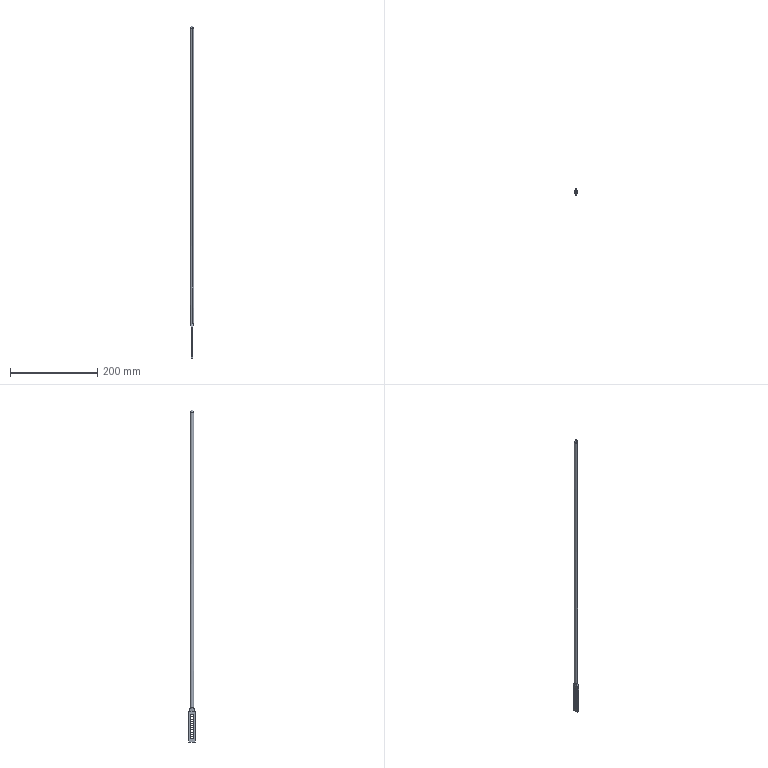Part | STEP file | _X2_751F4E45_X0_LG003_X2_8-1054 | 1 solid | 34 faces | box 8.003 x 14 x 760 mm | volume 36967 mm3 | cylinder 22 | plane 6 | spline 4 | cone 2 | commonest cylinder face diameters 6.1 x20 8 x2